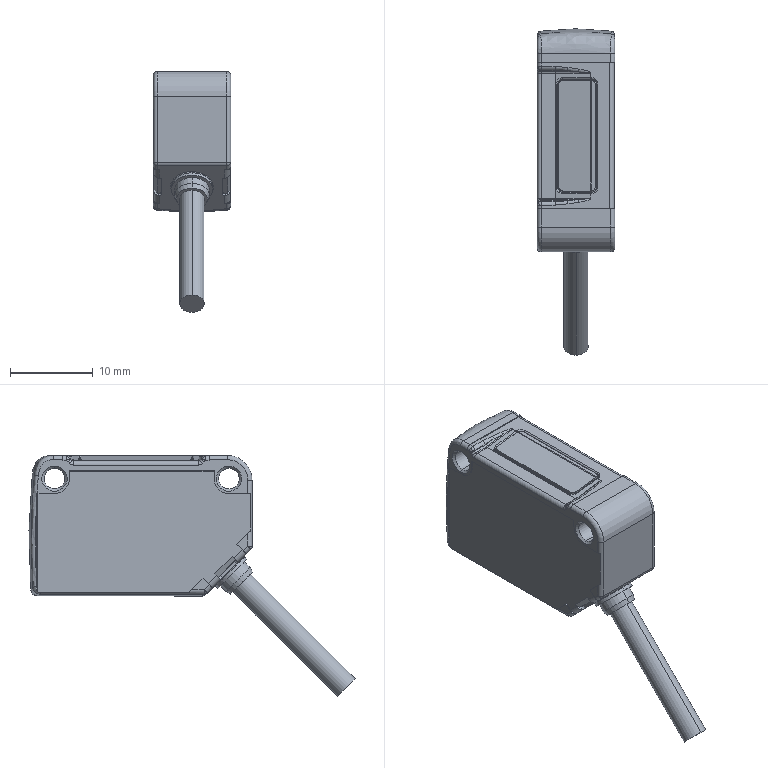Part | STEP file | LR-XH50-Part-1-4 | 1 solid | 216 faces | box 9.4 x 39.451 x 29.153 mm | volume 4011 mm3 | cylinder 87 | plane 61 | spline 21 | torus 18 | sphere 15 | cone 14 | commonest cylinder face diameters 1 x32 0.3 x11 0.4 x11 3 x6 0.6 x4 1.2 x4